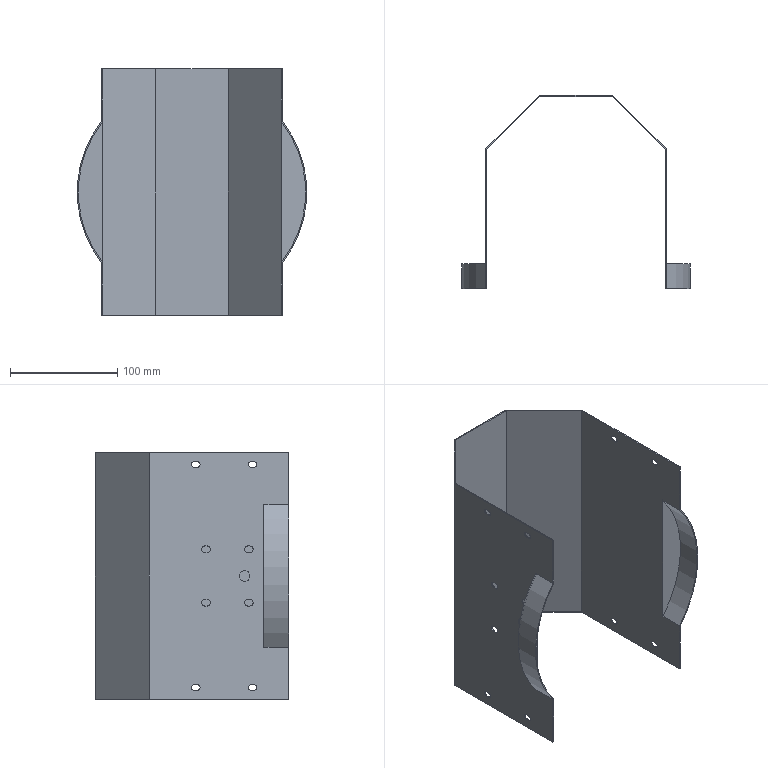Part | SolidWorks | features BaseBody 1 | 1 solid | 72 faces | box 214 x 180 x 230 mm | volume 111689 mm3 | plane 42 | cylinder 30 | commonest cylinder face diameters 5 x16 6 x8 10 x2 212 x2 214 x2